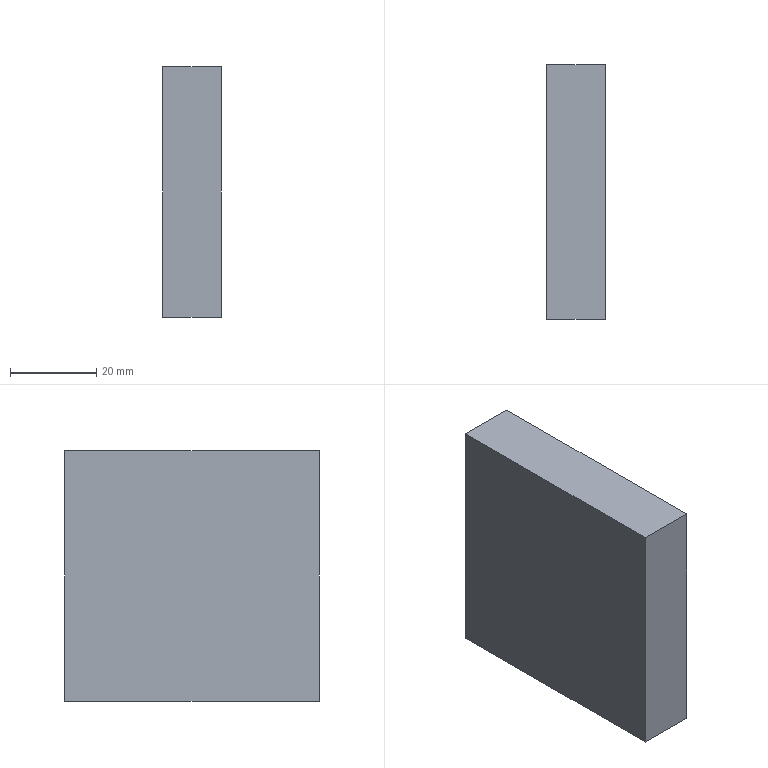Part | SolidWorks | features BaseBody 1 | 1 solid | 6 faces | box 13.5 x 59 x 58 mm | volume 46197 mm3 | plane 6
STEP:
#1=CARTESIAN_POINT('',(13.5,0.,-58.));
#2=VERTEX_POINT('',#1);
#3=CARTESIAN_POINT('',(13.5,0.,0.));
#4=VERTEX_POINT('',#3);
#5=CARTESIAN_POINT('',(13.5,0.,0.));
#6=DIRECTION('',(0.,0.,1.));
#7=VECTOR('',#6,1000.);
#8=LINE('',#5,#7);
#9=EDGE_CURVE('',#2,#4,#8,.T.);
#10=ORIENTED_EDGE('',*,*,#9,.F.);
#11=CARTESIAN_POINT('',(13.5,59.,-58.));
#12=VERTEX_POINT('',#11);
#13=CARTESIAN_POINT('',(13.5,0.,-58.));
#14=DIRECTION('',(0.,-1.,0.));
#15=VECTOR('',#14,1000.);
#16=LINE('',#13,#15);
#17=EDGE_CURVE('',#12,#2,#16,.T.);
#18=ORIENTED_EDGE('',*,*,#17,.F.);
#19=CARTESIAN_POINT('',(13.5,59.,0.));
#20=VERTEX_POINT('',#19);
#21=CARTESIAN_POINT('',(13.5,59.,0.));
#22=DIRECTION('',(0.,0.,-1.));
#23=VECTOR('',#22,1000.);
#24=LINE('',#21,#23);
#25=EDGE_CURVE('',#20,#12,#24,.T.);
#26=ORIENTED_EDGE('',*,*,#25,.F.);
#27=CARTESIAN_POINT('',(13.5,0.,0.));
#28=DIRECTION('',(0.,1.,0.));
#29=VECTOR('',#28,1000.);
#30=LINE('',#27,#29);
#31=EDGE_CURVE('',#4,#20,#30,.T.);
#32=ORIENTED_EDGE('',*,*,#31,.F.);
#33=EDGE_LOOP('',(#10,#18,#26,#32));
#34=FACE_OUTER_BOUND('',#33,.T.);
#35=CARTESIAN_POINT('',(13.5,0.,0.));
#36=DIRECTION('',(-1.,0.,0.));
#37=DIRECTION('',(0.,0.,1.));
#38=AXIS2_PLACEMENT_3D('',#35,#36,#37);
#39=PLANE('',#38);
#40=ADVANCED_FACE('',(#34),#39,.F.);
#41=CARTESIAN_POINT('',(0.,0.,0.));
#42=VERTEX_POINT('',#41);
#43=CARTESIAN_POINT('',(13.5,0.,0.));
#44=DIRECTION('',(-1.,0.,0.));
#45=VECTOR('',#44,1000.);
#46=LINE('',#43,#45);
#47=EDGE_CURVE('',#4,#42,#46,.T.);
#48=ORIENTED_EDGE('',*,*,#47,.F.);
#49=ORIENTED_EDGE('',*,*,#31,.T.);
#50=CARTESIAN_POINT('',(0.,59.,0.));
#51=VERTEX_POINT('',#50);
#52=CARTESIAN_POINT('',(13.5,59.,0.));
#53=DIRECTION('',(1.,0.,0.));
#54=VECTOR('',#53,1000.);
#55=LINE('',#52,#54);
#56=EDGE_CURVE('',#51,#20,#55,.T.);
#57=ORIENTED_EDGE('',*,*,#56,.F.);
#58=CARTESIAN_POINT('',(0.,0.,0.));
#59=DIRECTION('',(0.,1.,0.));
#60=VECTOR('',#59,1000.);
#61=LINE('',#58,#60);
#62=EDGE_CURVE('',#42,#51,#61,.T.);
#63=ORIENTED_EDGE('',*,*,#62,.F.);
#64=EDGE_LOOP('',(#48,#49,#57,#63));
#65=FACE_OUTER_BOUND('',#64,.T.);
#66=CARTESIAN_POINT('',(13.5,0.,0.));
#67=DIRECTION('',(0.,0.,-1.));
#68=DIRECTION('',(-1.,0.,0.));
#69=AXIS2_PLACEMENT_3D('',#66,#67,#68);
#70=PLANE('',#69);
#71=ADVANCED_FACE('',(#65),#70,.F.);
#72=CARTESIAN_POINT('',(0.,0.,-58.));
#73=VERTEX_POINT('',#72);
#74=CARTESIAN_POINT('',(13.5,0.,-58.));
#75=DIRECTION('',(-1.,0.,0.));
#76=VECTOR('',#75,1000.);
#77=LINE('',#74,#76);
#78=EDGE_CURVE('',#2,#73,#77,.T.);
#79=ORIENTED_EDGE('',*,*,#78,.F.);
#80=ORIENTED_EDGE('',*,*,#9,.T.);
#81=ORIENTED_EDGE('',*,*,#47,.T.);
#82=CARTESIAN_POINT('',(0.,0.,0.));
#83=DIRECTION('',(0.,0.,1.));
#84=VECTOR('',#83,1000.);
#85=LINE('',#82,#84);
#86=EDGE_CURVE('',#73,#42,#85,.T.);
#87=ORIENTED_EDGE('',*,*,#86,.F.);
#88=EDGE_LOOP('',(#79,#80,#81,#87));
#89=FACE_OUTER_BOUND('',#88,.T.);
#90=CARTESIAN_POINT('',(13.5,0.,0.));
#91=DIRECTION('',(0.,1.,0.));
#92=DIRECTION('',(0.,0.,1.));
#93=AXIS2_PLACEMENT_3D('',#90,#91,#92);
#94=PLANE('',#93);
#95=ADVANCED_FACE('',(#89),#94,.F.);
#96=CARTESIAN_POINT('',(0.,59.,-58.));
#97=VERTEX_POINT('',#96);
#98=CARTESIAN_POINT('',(13.5,59.,-58.));
#99=DIRECTION('',(-1.,0.,0.));
#100=VECTOR('',#99,1000.);
#101=LINE('',#98,#100);
#102=EDGE_CURVE('',#12,#97,#101,.T.);
#103=ORIENTED_EDGE('',*,*,#102,.F.);
#104=ORIENTED_EDGE('',*,*,#17,.T.);
#105=ORIENTED_EDGE('',*,*,#78,.T.);
#106=CARTESIAN_POINT('',(0.,0.,-58.));
#107=DIRECTION('',(0.,-1.,0.));
#108=VECTOR('',#107,1000.);
#109=LINE('',#106,#108);
#110=EDGE_CURVE('',#97,#73,#109,.T.);
#111=ORIENTED_EDGE('',*,*,#110,.F.);
#112=EDGE_LOOP('',(#103,#104,#105,#111));
#113=FACE_OUTER_BOUND('',#112,.T.);
#114=CARTESIAN_POINT('',(13.5,0.,-58.));
#115=DIRECTION('',(0.,0.,1.));
#116=DIRECTION('',(1.,0.,0.));
#117=AXIS2_PLACEMENT_3D('',#114,#115,#116);
#118=PLANE('',#117);
#119=ADVANCED_FACE('',(#113),#118,.F.);
#120=ORIENTED_EDGE('',*,*,#56,.T.);
#121=ORIENTED_EDGE('',*,*,#25,.T.);
#122=ORIENTED_EDGE('',*,*,#102,.T.);
#123=CARTESIAN_POINT('',(0.,59.,0.));
#124=DIRECTION('',(0.,0.,-1.));
#125=VECTOR('',#124,1000.);
#126=LINE('',#123,#125);
#127=EDGE_CURVE('',#51,#97,#126,.T.);
#128=ORIENTED_EDGE('',*,*,#127,.F.);
#129=EDGE_LOOP('',(#120,#121,#122,#128));
#130=FACE_OUTER_BOUND('',#129,.T.);
#131=CARTESIAN_POINT('',(13.5,59.,0.));
#132=DIRECTION('',(0.,-1.,0.));
#133=DIRECTION('',(0.,0.,-1.));
#134=AXIS2_PLACEMENT_3D('',#131,#132,#133);
#135=PLANE('',#134);
#136=ADVANCED_FACE('',(#130),#135,.F.);
#137=ORIENTED_EDGE('',*,*,#110,.T.);
#138=ORIENTED_EDGE('',*,*,#86,.T.);
#139=ORIENTED_EDGE('',*,*,#62,.T.);
#140=ORIENTED_EDGE('',*,*,#127,.T.);
#141=EDGE_LOOP('',(#137,#138,#139,#140));
#142=FACE_OUTER_BOUND('',#141,.T.);
#143=CARTESIAN_POINT('',(0.,0.,0.));
#144=DIRECTION('',(-1.,0.,0.));
#145=DIRECTION('',(0.,0.,1.));
#146=AXIS2_PLACEMENT_3D('',#143,#144,#145);
#147=PLANE('',#146);
#148=ADVANCED_FACE('',(#142),#147,.T.);
#149=CLOSED_SHELL('',(#40,#71,#95,#119,#136,#148));
#150=MANIFOLD_SOLID_BREP('',#149);
#151=CARTESIAN_POINT('',(0.,0.,0.));
#152=DIRECTION('',(0.,0.,1.));
#153=DIRECTION('',(1.,0.,0.));
#154=AXIS2_PLACEMENT_3D('',#151,#152,#153);
#155=(LENGTH_UNIT()NAMED_UNIT(*)SI_UNIT(.MILLI.,.METRE.));
#156=UNCERTAINTY_MEASURE_WITH_UNIT(LENGTH_MEASURE(0.00001),#155,'','');
#157=(NAMED_UNIT(*)PLANE_ANGLE_UNIT()SI_UNIT($,.RADIAN.));
#158=(NAMED_UNIT(*)SI_UNIT($,.STERADIAN.)SOLID_ANGLE_UNIT());
#159=(GEOMETRIC_REPRESENTATION_CONTEXT(3)GLOBAL_UNCERTAINTY_ASSIGNED_CONTEXT((#156))GLOBAL_UNIT_ASSIGNED_CONTEXT((#155,#157,#158))REPRESENTATION_CONTEXT('',''));
#160=ADVANCED_BREP_SHAPE_REPRESENTATION('',(#150,#154),#159);